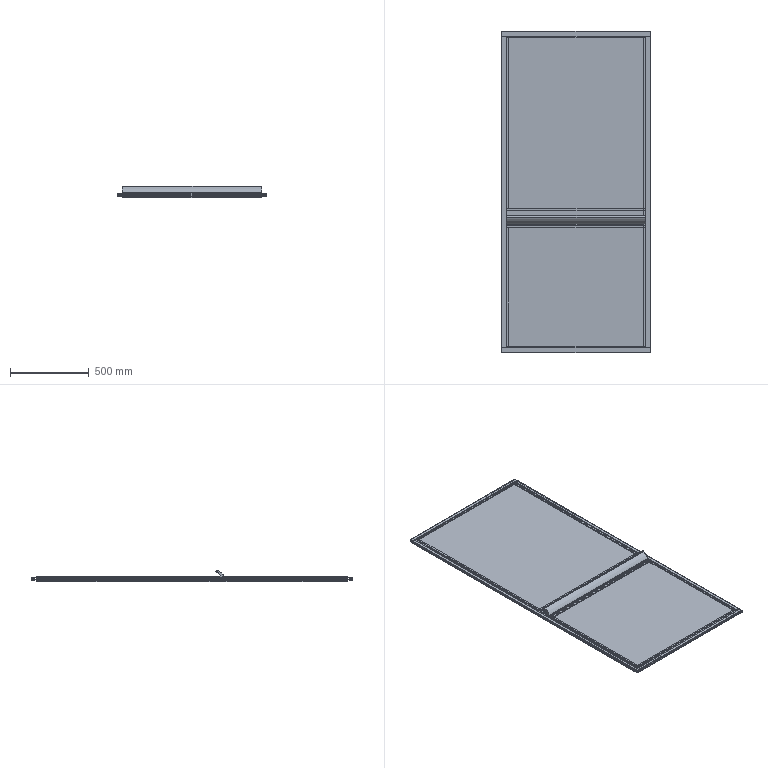Part | 22 solids | 546 faces | box 940 x 2036 x 71.386 mm | volume 40242379 mm3 | plane 390 | cylinder 156 | commonest cylinder face diameters 1.1 x36 3.6 x32 5.8 x29 4 x24 1 x10 0.4 x8